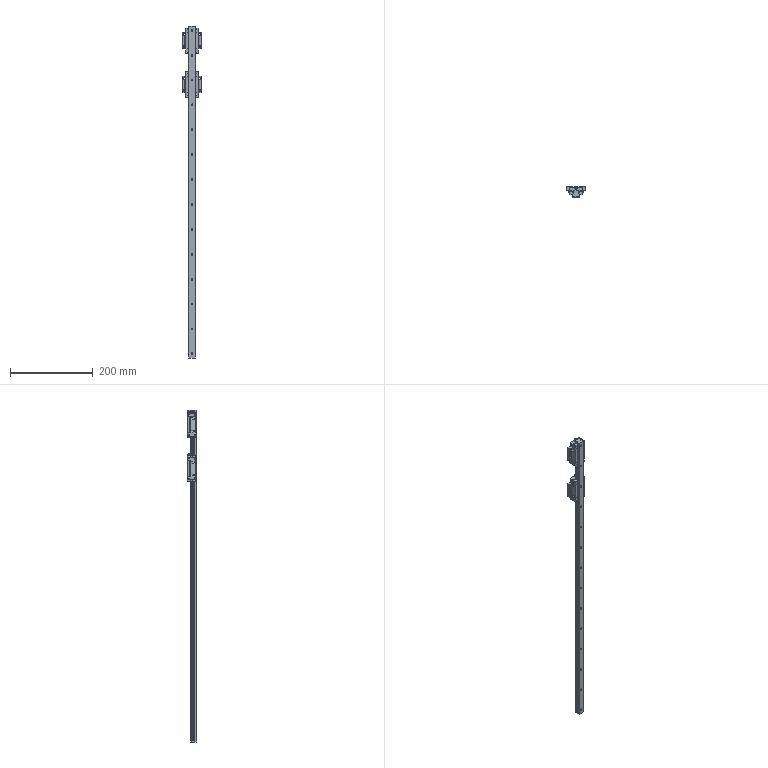Part | SolidWorks | 13 solids | 1678 faces | box 47 x 24.01 x 800.23 mm | volume 223806 mm3 | plane 1152 | spline 238 | cylinder 222 | torus 32 | sphere 20 | cone 14 | commonest cylinder face diameters 1.459 x66 4.5 x28 7.5 x28 3.15 x24 5 x20 0.425 x16